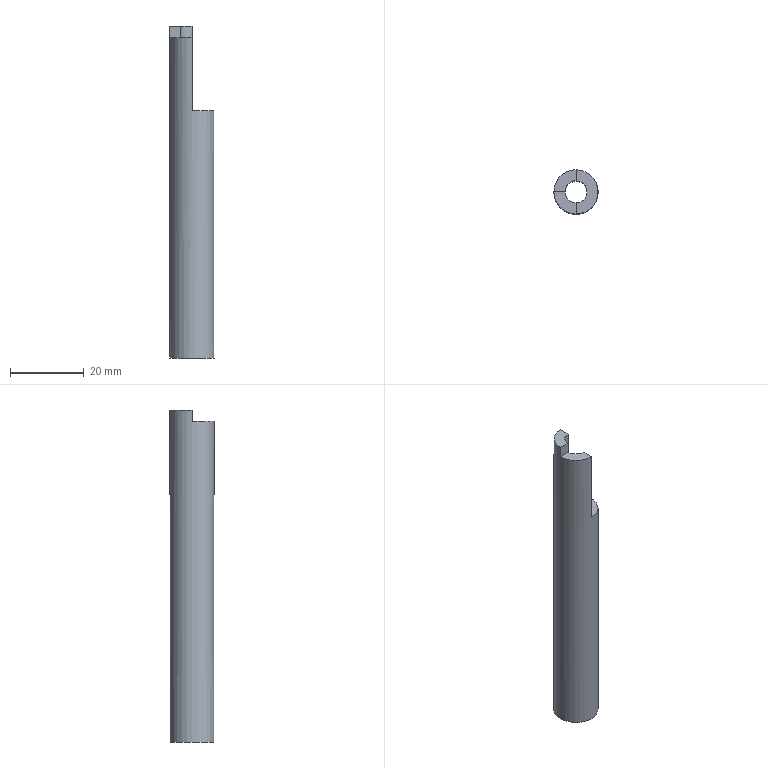Part | NX | features solid 2 | 1 solid | 9 faces | box 12 x 12 x 90 mm | volume 6593 mm3 | plane 7 | cylinder 2 | commonest cylinder face diameters 6.003 x1 12 x1
STEP:
#1=CARTESIAN_POINT('',(3145.094,-894.124,838.716));
#2=VERTEX_POINT('',#1);
#3=CARTESIAN_POINT('',(3145.094,-897.123,838.716));
#4=VERTEX_POINT('',#3);
#5=CARTESIAN_POINT('',(3145.094,-891.123,838.716));
#6=DIRECTION('',(0.,-1.,0.));
#7=VECTOR('',#6,1000.);
#8=LINE('',#5,#7);
#9=EDGE_CURVE('',#2,#4,#8,.T.);
#10=ORIENTED_EDGE('',*,*,#9,.T.);
#11=CARTESIAN_POINT('',(3145.094,-897.123,818.716));
#12=VERTEX_POINT('',#11);
#13=CARTESIAN_POINT('',(3145.094,-897.123,841.716));
#14=DIRECTION('',(0.,0.,-1.));
#15=VECTOR('',#14,1000.);
#16=LINE('',#13,#15);
#17=EDGE_CURVE('',#4,#12,#16,.T.);
#18=ORIENTED_EDGE('',*,*,#17,.T.);
#19=CARTESIAN_POINT('',(3145.094,-894.124,818.716));
#20=VERTEX_POINT('',#19);
#21=CARTESIAN_POINT('',(3145.094,-879.123,818.716));
#22=DIRECTION('',(0.,-1.,0.));
#23=VECTOR('',#22,1000.);
#24=LINE('',#21,#23);
#25=EDGE_CURVE('',#12,#20,#24,.F.);
#26=ORIENTED_EDGE('',*,*,#25,.T.);
#27=CARTESIAN_POINT('',(3145.094,-894.124,841.716));
#28=DIRECTION('',(0.,0.,-1.));
#29=VECTOR('',#28,1000.);
#30=LINE('',#27,#29);
#31=EDGE_CURVE('',#2,#20,#30,.T.);
#32=ORIENTED_EDGE('',*,*,#31,.F.);
#33=EDGE_LOOP('',(#10,#18,#26,#32));
#34=FACE_BOUND('',#33,.T.);
#35=CARTESIAN_POINT('',(3145.094,-879.123,818.716));
#36=DIRECTION('',(-1.,0.,0.));
#37=DIRECTION('',(0.,0.,1.));
#38=AXIS2_PLACEMENT_3D('',#35,#36,#37);
#39=PLANE('',#38);
#40=ADVANCED_FACE('',(#34),#39,.F.);
#41=CARTESIAN_POINT('',(3142.092,-891.123,751.716));
#42=VERTEX_POINT('',#41);
#43=CARTESIAN_POINT('',(3145.094,-891.123,751.716));
#44=DIRECTION('',(0.,0.,-1.));
#45=DIRECTION('',(-1.,0.,0.));
#46=AXIS2_PLACEMENT_3D('',#43,#44,#45);
#47=CIRCLE('',#46,3.002);
#48=EDGE_CURVE('',#42,#42,#47,.F.);
#49=ORIENTED_EDGE('',*,*,#48,.T.);
#50=EDGE_LOOP('',(#49));
#51=FACE_BOUND('',#50,.T.);
#52=CARTESIAN_POINT('',(3139.094,-891.123,751.716));
#53=VERTEX_POINT('',#52);
#54=CARTESIAN_POINT('',(3145.094,-891.123,751.716));
#55=DIRECTION('',(0.,0.,-1.));
#56=DIRECTION('',(-1.,0.,0.));
#57=AXIS2_PLACEMENT_3D('',#54,#55,#56);
#58=CIRCLE('',#57,6.);
#59=EDGE_CURVE('',#53,#53,#58,.F.);
#60=ORIENTED_EDGE('',*,*,#59,.F.);
#61=EDGE_LOOP('',(#60));
#62=FACE_BOUND('',#61,.T.);
#63=CARTESIAN_POINT('',(3145.094,-891.123,751.716));
#64=DIRECTION('',(0.,0.,-1.));
#65=DIRECTION('',(-1.,0.,0.));
#66=AXIS2_PLACEMENT_3D('',#63,#64,#65);
#67=PLANE('',#66);
#68=ADVANCED_FACE('',(#51,#62),#67,.T.);
#69=CARTESIAN_POINT('',(3142.092,-891.123,841.716));
#70=VERTEX_POINT('',#69);
#71=CARTESIAN_POINT('',(3139.094,-891.123,841.716));
#72=VERTEX_POINT('',#71);
#73=CARTESIAN_POINT('',(3145.094,-891.123,841.716));
#74=DIRECTION('',(-1.,0.,0.));
#75=VECTOR('',#74,1000.);
#76=LINE('',#73,#75);
#77=EDGE_CURVE('',#70,#72,#76,.T.);
#78=ORIENTED_EDGE('',*,*,#77,.F.);
#79=CARTESIAN_POINT('',(3145.094,-888.121,841.716));
#80=VERTEX_POINT('',#79);
#81=CARTESIAN_POINT('',(3145.094,-891.123,841.716));
#82=DIRECTION('',(0.,0.,-1.));
#83=DIRECTION('',(1.,0.,0.));
#84=AXIS2_PLACEMENT_3D('',#81,#82,#83);
#85=CIRCLE('',#84,3.002);
#86=EDGE_CURVE('',#70,#80,#85,.T.);
#87=ORIENTED_EDGE('',*,*,#86,.T.);
#88=CARTESIAN_POINT('',(3145.094,-885.123,841.716));
#89=VERTEX_POINT('',#88);
#90=CARTESIAN_POINT('',(3145.094,-879.123,841.716));
#91=DIRECTION('',(0.,-1.,0.));
#92=VECTOR('',#91,1000.);
#93=LINE('',#90,#92);
#94=EDGE_CURVE('',#89,#80,#93,.T.);
#95=ORIENTED_EDGE('',*,*,#94,.F.);
#96=CARTESIAN_POINT('',(3145.094,-891.123,841.716));
#97=DIRECTION('',(0.,0.,-1.));
#98=DIRECTION('',(1.,0.,0.));
#99=AXIS2_PLACEMENT_3D('',#96,#97,#98);
#100=CIRCLE('',#99,6.);
#101=EDGE_CURVE('',#72,#89,#100,.T.);
#102=ORIENTED_EDGE('',*,*,#101,.F.);
#103=EDGE_LOOP('',(#78,#87,#95,#102));
#104=FACE_BOUND('',#103,.T.);
#105=CARTESIAN_POINT('',(3145.094,-891.123,841.716));
#106=DIRECTION('',(0.,0.,1.));
#107=DIRECTION('',(1.,0.,0.));
#108=AXIS2_PLACEMENT_3D('',#105,#106,#107);
#109=PLANE('',#108);
#110=ADVANCED_FACE('',(#104),#109,.T.);
#111=CARTESIAN_POINT('',(3139.094,-891.123,838.716));
#112=VERTEX_POINT('',#111);
#113=CARTESIAN_POINT('',(3139.094,-891.123,841.716));
#114=DIRECTION('',(0.,0.,-1.));
#115=VECTOR('',#114,1000.);
#116=LINE('',#113,#115);
#117=EDGE_CURVE('',#72,#112,#116,.T.);
#118=ORIENTED_EDGE('',*,*,#117,.F.);
#119=ORIENTED_EDGE('',*,*,#101,.T.);
#120=CARTESIAN_POINT('',(3145.094,-885.123,818.716));
#121=VERTEX_POINT('',#120);
#122=CARTESIAN_POINT('',(3145.094,-885.123,841.716));
#123=DIRECTION('',(0.,0.,-1.));
#124=VECTOR('',#123,1000.);
#125=LINE('',#122,#124);
#126=EDGE_CURVE('',#121,#89,#125,.F.);
#127=ORIENTED_EDGE('',*,*,#126,.F.);
#128=CARTESIAN_POINT('',(3145.094,-891.123,818.716));
#129=DIRECTION('',(0.,0.,-1.));
#130=DIRECTION('',(-1.,0.,0.));
#131=AXIS2_PLACEMENT_3D('',#128,#129,#130);
#132=CIRCLE('',#131,6.);
#133=EDGE_CURVE('',#12,#121,#132,.F.);
#134=ORIENTED_EDGE('',*,*,#133,.F.);
#135=ORIENTED_EDGE('',*,*,#17,.F.);
#136=CARTESIAN_POINT('',(3145.094,-891.123,838.716));
#137=DIRECTION('',(0.,0.,1.));
#138=DIRECTION('',(1.,0.,0.));
#139=AXIS2_PLACEMENT_3D('',#136,#137,#138);
#140=CIRCLE('',#139,6.);
#141=EDGE_CURVE('',#4,#112,#140,.F.);
#142=ORIENTED_EDGE('',*,*,#141,.T.);
#143=EDGE_LOOP('',(#118,#119,#127,#134,#135,#142));
#144=FACE_BOUND('',#143,.T.);
#145=ORIENTED_EDGE('',*,*,#59,.T.);
#146=EDGE_LOOP('',(#145));
#147=FACE_BOUND('',#146,.T.);
#148=CARTESIAN_POINT('',(3145.094,-891.123,841.716));
#149=DIRECTION('',(0.,0.,-1.));
#150=DIRECTION('',(1.,0.,0.));
#151=AXIS2_PLACEMENT_3D('',#148,#149,#150);
#152=CYLINDRICAL_SURFACE('',#151,6.);
#153=ADVANCED_FACE('',(#144,#147),#152,.T.);
#154=ORIENTED_EDGE('',*,*,#48,.F.);
#155=EDGE_LOOP('',(#154));
#156=FACE_BOUND('',#155,.T.);
#157=ORIENTED_EDGE('',*,*,#86,.F.);
#158=CARTESIAN_POINT('',(3142.092,-891.123,838.716));
#159=VERTEX_POINT('',#158);
#160=CARTESIAN_POINT('',(3142.092,-891.123,841.716));
#161=DIRECTION('',(0.,0.,-1.));
#162=VECTOR('',#161,1000.);
#163=LINE('',#160,#162);
#164=EDGE_CURVE('',#70,#159,#163,.T.);
#165=ORIENTED_EDGE('',*,*,#164,.T.);
#166=CARTESIAN_POINT('',(3145.094,-891.123,838.716));
#167=DIRECTION('',(0.,0.,1.));
#168=DIRECTION('',(1.,0.,0.));
#169=AXIS2_PLACEMENT_3D('',#166,#167,#168);
#170=CIRCLE('',#169,3.002);
#171=EDGE_CURVE('',#2,#159,#170,.F.);
#172=ORIENTED_EDGE('',*,*,#171,.F.);
#173=ORIENTED_EDGE('',*,*,#31,.T.);
#174=CARTESIAN_POINT('',(3145.094,-888.121,818.716));
#175=VERTEX_POINT('',#174);
#176=CARTESIAN_POINT('',(3145.094,-891.123,818.716));
#177=DIRECTION('',(0.,0.,-1.));
#178=DIRECTION('',(-1.,0.,0.));
#179=AXIS2_PLACEMENT_3D('',#176,#177,#178);
#180=CIRCLE('',#179,3.002);
#181=EDGE_CURVE('',#20,#175,#180,.F.);
#182=ORIENTED_EDGE('',*,*,#181,.T.);
#183=CARTESIAN_POINT('',(3145.094,-888.121,841.716));
#184=DIRECTION('',(0.,0.,-1.));
#185=VECTOR('',#184,1000.);
#186=LINE('',#183,#185);
#187=EDGE_CURVE('',#175,#80,#186,.F.);
#188=ORIENTED_EDGE('',*,*,#187,.T.);
#189=EDGE_LOOP('',(#157,#165,#172,#173,#182,#188));
#190=FACE_BOUND('',#189,.T.);
#191=CARTESIAN_POINT('',(3145.094,-891.123,841.716));
#192=DIRECTION('',(0.,0.,-1.));
#193=DIRECTION('',(1.,0.,0.));
#194=AXIS2_PLACEMENT_3D('',#191,#192,#193);
#195=CYLINDRICAL_SURFACE('',#194,3.002);
#196=ADVANCED_FACE('',(#156,#190),#195,.F.);
#197=ORIENTED_EDGE('',*,*,#126,.T.);
#198=ORIENTED_EDGE('',*,*,#94,.T.);
#199=ORIENTED_EDGE('',*,*,#187,.F.);
#200=CARTESIAN_POINT('',(3145.094,-879.123,818.716));
#201=DIRECTION('',(0.,-1.,0.));
#202=VECTOR('',#201,1000.);
#203=LINE('',#200,#202);
#204=EDGE_CURVE('',#175,#121,#203,.F.);
#205=ORIENTED_EDGE('',*,*,#204,.T.);
#206=EDGE_LOOP('',(#197,#198,#199,#205));
#207=FACE_BOUND('',#206,.T.);
#208=CARTESIAN_POINT('',(3145.094,-879.123,818.716));
#209=DIRECTION('',(-1.,0.,0.));
#210=DIRECTION('',(0.,0.,1.));
#211=AXIS2_PLACEMENT_3D('',#208,#209,#210);
#212=PLANE('',#211);
#213=ADVANCED_FACE('',(#207),#212,.F.);
#214=ORIENTED_EDGE('',*,*,#133,.T.);
#215=ORIENTED_EDGE('',*,*,#204,.F.);
#216=ORIENTED_EDGE('',*,*,#181,.F.);
#217=ORIENTED_EDGE('',*,*,#25,.F.);
#218=EDGE_LOOP('',(#214,#215,#216,#217));
#219=FACE_BOUND('',#218,.T.);
#220=CARTESIAN_POINT('',(-444.,5.,818.716));
#221=DIRECTION('',(0.,0.,-1.));
#222=DIRECTION('',(-1.,0.,0.));
#223=AXIS2_PLACEMENT_3D('',#220,#221,#222);
#224=PLANE('',#223);
#225=ADVANCED_FACE('',(#219),#224,.F.);
#226=ORIENTED_EDGE('',*,*,#117,.T.);
#227=CARTESIAN_POINT('',(3145.094,-891.123,838.716));
#228=DIRECTION('',(-1.,0.,0.));
#229=VECTOR('',#228,1000.);
#230=LINE('',#227,#229);
#231=EDGE_CURVE('',#112,#159,#230,.F.);
#232=ORIENTED_EDGE('',*,*,#231,.T.);
#233=ORIENTED_EDGE('',*,*,#164,.F.);
#234=ORIENTED_EDGE('',*,*,#77,.T.);
#235=EDGE_LOOP('',(#226,#232,#233,#234));
#236=FACE_BOUND('',#235,.T.);
#237=CARTESIAN_POINT('',(3145.094,-891.123,838.716));
#238=DIRECTION('',(0.,1.,0.));
#239=DIRECTION('',(0.,0.,1.));
#240=AXIS2_PLACEMENT_3D('',#237,#238,#239);
#241=PLANE('',#240);
#242=ADVANCED_FACE('',(#236),#241,.F.);
#243=ORIENTED_EDGE('',*,*,#9,.F.);
#244=ORIENTED_EDGE('',*,*,#171,.T.);
#245=ORIENTED_EDGE('',*,*,#231,.F.);
#246=ORIENTED_EDGE('',*,*,#141,.F.);
#247=EDGE_LOOP('',(#243,#244,#245,#246));
#248=FACE_BOUND('',#247,.T.);
#249=CARTESIAN_POINT('',(-444.,5.,838.716));
#250=DIRECTION('',(0.,0.,1.));
#251=DIRECTION('',(1.,0.,0.));
#252=AXIS2_PLACEMENT_3D('',#249,#250,#251);
#253=PLANE('',#252);
#254=ADVANCED_FACE('',(#248),#253,.T.);
#255=CLOSED_SHELL('',(#40,#68,#110,#153,#196,#213,#225,#242,#254));
#256=MANIFOLD_SOLID_BREP('',#255);
#257=(LENGTH_UNIT()NAMED_UNIT(*)SI_UNIT(.MILLI.,.METRE.));
#258=UNCERTAINTY_MEASURE_WITH_UNIT(LENGTH_MEASURE(0.00001),#257,'','');
#259=(NAMED_UNIT(*)PLANE_ANGLE_UNIT()SI_UNIT($,.RADIAN.));
#260=(NAMED_UNIT(*)SI_UNIT($,.STERADIAN.)SOLID_ANGLE_UNIT());
#261=(GEOMETRIC_REPRESENTATION_CONTEXT(3)GLOBAL_UNCERTAINTY_ASSIGNED_CONTEXT((#258))GLOBAL_UNIT_ASSIGNED_CONTEXT((#257,#259,#260))REPRESENTATION_CONTEXT('',''));
#262=ADVANCED_BREP_SHAPE_REPRESENTATION('',(#256),#261);